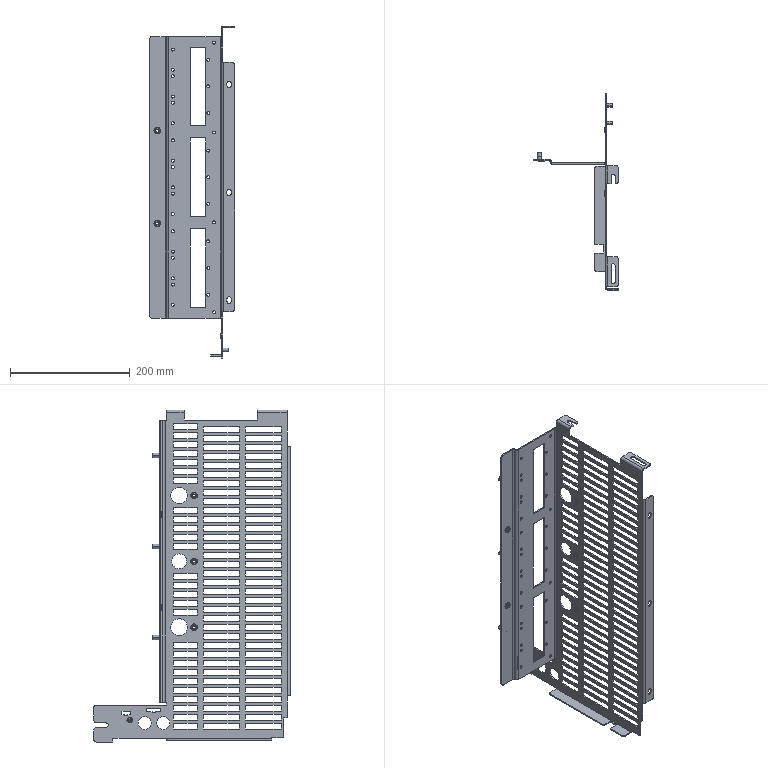Part | STEP file | 64633091_AF0 | 1 solid | 707 faces | box 142 x 328 x 554.508 mm | volume 249746 mm3 | plane 516 | cylinder 155 | torus 36 | commonest cylinder face diameters 5 x64 8 x21 7 x15 4 x13 9 x10 4.8 x8